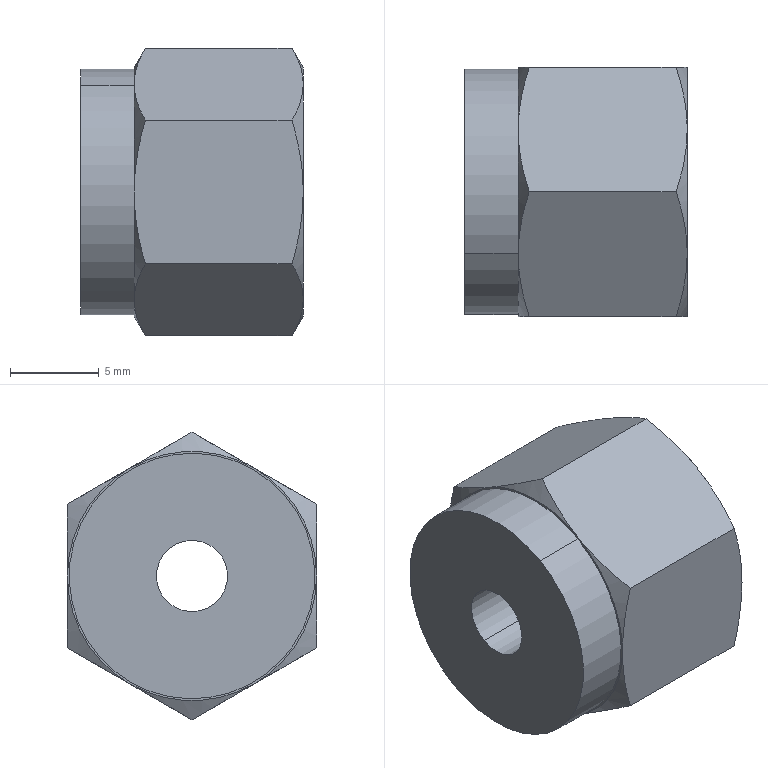Part | STEP file | SKTGK4-1-Part-1-7 | 1 solid | 28 faces | box 12.5 x 14 x 16.166 mm | volume 1459 mm3 | cone 12 | plane 10 | cylinder 6 | commonest cylinder face diameters 4 x2 11.112 x2 13.8 x2
STEP:
#1=CARTESIAN_POINT('',(7.3,9.778,3.271));
#2=VERTEX_POINT('',#1);
#3=CARTESIAN_POINT('',(7.3,4.222,12.895));
#4=VERTEX_POINT('',#3);
#5=CARTESIAN_POINT('',(7.3,7.,8.083));
#6=DIRECTION('',(1.,0.,0.));
#7=DIRECTION('',(0.,-0.5,0.866));
#8=AXIS2_PLACEMENT_3D('',#5,#6,#7);
#9=CIRCLE('',#8,5.556);
#10=EDGE_CURVE('',#2,#4,#9,.T.);
#11=ORIENTED_EDGE('',*,*,#10,.F.);
#12=CARTESIAN_POINT('',(12.5,9.778,3.271));
#13=VERTEX_POINT('',#12);
#14=CARTESIAN_POINT('',(12.5,9.778,3.271));
#15=DIRECTION('',(1.,0.,0.));
#16=VECTOR('',#15,1000.);
#17=LINE('',#14,#16);
#18=EDGE_CURVE('',#2,#13,#17,.T.);
#19=ORIENTED_EDGE('',*,*,#18,.T.);
#20=CARTESIAN_POINT('',(12.5,4.222,12.895));
#21=VERTEX_POINT('',#20);
#22=CARTESIAN_POINT('',(12.5,7.,8.083));
#23=DIRECTION('',(1.,0.,0.));
#24=DIRECTION('',(0.,-0.5,0.866));
#25=AXIS2_PLACEMENT_3D('',#22,#23,#24);
#26=CIRCLE('',#25,5.556);
#27=EDGE_CURVE('',#13,#21,#26,.T.);
#28=ORIENTED_EDGE('',*,*,#27,.T.);
#29=CARTESIAN_POINT('',(12.5,4.222,12.895));
#30=DIRECTION('',(1.,0.,0.));
#31=VECTOR('',#30,1000.);
#32=LINE('',#29,#31);
#33=EDGE_CURVE('',#4,#21,#32,.T.);
#34=ORIENTED_EDGE('',*,*,#33,.F.);
#35=EDGE_LOOP('',(#11,#19,#28,#34));
#36=FACE_OUTER_BOUND('',#35,.T.);
#37=CARTESIAN_POINT('',(12.5,7.,8.083));
#38=DIRECTION('',(1.,0.,0.));
#39=DIRECTION('',(0.,-0.5,0.866));
#40=AXIS2_PLACEMENT_3D('',#37,#38,#39);
#41=CYLINDRICAL_SURFACE('',#40,5.556);
#42=ADVANCED_FACE('',(#36),#41,.F.);
#43=CARTESIAN_POINT('',(0.,8.,6.351));
#44=VERTEX_POINT('',#43);
#45=CARTESIAN_POINT('',(0.,6.,9.815));
#46=VERTEX_POINT('',#45);
#47=CARTESIAN_POINT('',(0.,7.,8.083));
#48=DIRECTION('',(1.,0.,0.));
#49=DIRECTION('',(0.,-0.5,0.866));
#50=AXIS2_PLACEMENT_3D('',#47,#48,#49);
#51=CIRCLE('',#50,2.);
#52=EDGE_CURVE('',#44,#46,#51,.T.);
#53=ORIENTED_EDGE('',*,*,#52,.F.);
#54=CARTESIAN_POINT('',(7.3,8.,6.351));
#55=VERTEX_POINT('',#54);
#56=CARTESIAN_POINT('',(12.5,8.,6.351));
#57=DIRECTION('',(1.,0.,0.));
#58=VECTOR('',#57,1000.);
#59=LINE('',#56,#58);
#60=EDGE_CURVE('',#44,#55,#59,.T.);
#61=ORIENTED_EDGE('',*,*,#60,.T.);
#62=CARTESIAN_POINT('',(7.3,6.,9.815));
#63=VERTEX_POINT('',#62);
#64=CARTESIAN_POINT('',(7.3,7.,8.083));
#65=DIRECTION('',(1.,0.,0.));
#66=DIRECTION('',(0.,-0.5,0.866));
#67=AXIS2_PLACEMENT_3D('',#64,#65,#66);
#68=CIRCLE('',#67,2.);
#69=EDGE_CURVE('',#55,#63,#68,.T.);
#70=ORIENTED_EDGE('',*,*,#69,.T.);
#71=CARTESIAN_POINT('',(12.5,6.,9.815));
#72=DIRECTION('',(1.,0.,0.));
#73=VECTOR('',#72,1000.);
#74=LINE('',#71,#73);
#75=EDGE_CURVE('',#46,#63,#74,.T.);
#76=ORIENTED_EDGE('',*,*,#75,.F.);
#77=EDGE_LOOP('',(#53,#61,#70,#76));
#78=FACE_OUTER_BOUND('',#77,.T.);
#79=CARTESIAN_POINT('',(12.5,7.,8.083));
#80=DIRECTION('',(1.,0.,0.));
#81=DIRECTION('',(0.,-0.5,0.866));
#82=AXIS2_PLACEMENT_3D('',#79,#80,#81);
#83=CYLINDRICAL_SURFACE('',#82,2.);
#84=ADVANCED_FACE('',(#78),#83,.F.);
#85=CARTESIAN_POINT('',(0.,3.55,14.058));
#86=VERTEX_POINT('',#85);
#87=CARTESIAN_POINT('',(0.,10.45,2.107));
#88=VERTEX_POINT('',#87);
#89=CARTESIAN_POINT('',(0.,7.,8.083));
#90=DIRECTION('',(1.,0.,0.));
#91=DIRECTION('',(0.,-0.5,0.866));
#92=AXIS2_PLACEMENT_3D('',#89,#90,#91);
#93=CIRCLE('',#92,6.9);
#94=EDGE_CURVE('',#86,#88,#93,.T.);
#95=ORIENTED_EDGE('',*,*,#94,.T.);
#96=CARTESIAN_POINT('',(3.,10.45,2.107));
#97=VERTEX_POINT('',#96);
#98=CARTESIAN_POINT('',(12.5,10.45,2.107));
#99=DIRECTION('',(1.,0.,0.));
#100=VECTOR('',#99,1000.);
#101=LINE('',#98,#100);
#102=EDGE_CURVE('',#88,#97,#101,.T.);
#103=ORIENTED_EDGE('',*,*,#102,.T.);
#104=CARTESIAN_POINT('',(3.,3.55,14.058));
#105=VERTEX_POINT('',#104);
#106=CARTESIAN_POINT('',(3.,7.,8.083));
#107=DIRECTION('',(1.,0.,0.));
#108=DIRECTION('',(0.,-0.5,0.866));
#109=AXIS2_PLACEMENT_3D('',#106,#107,#108);
#110=CIRCLE('',#109,6.9);
#111=EDGE_CURVE('',#105,#97,#110,.T.);
#112=ORIENTED_EDGE('',*,*,#111,.F.);
#113=CARTESIAN_POINT('',(12.5,3.55,14.058));
#114=DIRECTION('',(1.,0.,0.));
#115=VECTOR('',#114,1000.);
#116=LINE('',#113,#115);
#117=EDGE_CURVE('',#86,#105,#116,.T.);
#118=ORIENTED_EDGE('',*,*,#117,.F.);
#119=EDGE_LOOP('',(#95,#103,#112,#118));
#120=FACE_OUTER_BOUND('',#119,.T.);
#121=CARTESIAN_POINT('',(12.5,7.,8.083));
#122=DIRECTION('',(1.,0.,0.));
#123=DIRECTION('',(0.,-0.5,0.866));
#124=AXIS2_PLACEMENT_3D('',#121,#122,#123);
#125=CYLINDRICAL_SURFACE('',#124,6.9);
#126=ADVANCED_FACE('',(#120),#125,.T.);
#127=CARTESIAN_POINT('',(11.875,14.,4.041));
#128=VERTEX_POINT('',#127);
#129=CARTESIAN_POINT('',(12.5,10.5,2.021));
#130=VERTEX_POINT('',#129);
#131=CARTESIAN_POINT('',(11.875,14.,4.041));
#132=CARTESIAN_POINT('',(12.255,12.86,3.383));
#133=CARTESIAN_POINT('',(12.5,11.699,2.713));
#134=CARTESIAN_POINT('',(12.5,10.5,2.021));
#135=B_SPLINE_CURVE_WITH_KNOTS('',3,(#131,#132,#133,#134),.UNSPECIFIED.,.F.,.F.,(4,4),(0.008823,0.01293),.UNSPECIFIED.);
#136=EDGE_CURVE('',#128,#130,#135,.T.);
#137=ORIENTED_EDGE('',*,*,#136,.F.);
#138=CARTESIAN_POINT('',(12.5,14.,8.083));
#139=VERTEX_POINT('',#138);
#140=CARTESIAN_POINT('',(12.5,14.,8.083));
#141=CARTESIAN_POINT('',(12.5,14.,7.74));
#142=CARTESIAN_POINT('',(12.485,14.,7.395));
#143=CARTESIAN_POINT('',(12.428,14.,6.714));
#144=CARTESIAN_POINT('',(12.386,14.,6.375));
#145=CARTESIAN_POINT('',(12.222,14.,5.366));
#146=CARTESIAN_POINT('',(12.065,14.,4.701));
#147=CARTESIAN_POINT('',(11.875,14.,4.041));
#148=B_SPLINE_CURVE_WITH_KNOTS('',3,(#140,#141,#142,#143,#144,#145,#146,#147),.UNSPECIFIED.,.F.,.F.,(4,2,2,4),(0.00409,0.005108,0.006127,0.008164),.UNSPECIFIED.);
#149=EDGE_CURVE('',#139,#128,#148,.T.);
#150=ORIENTED_EDGE('',*,*,#149,.F.);
#151=CARTESIAN_POINT('',(12.5,7.,8.083));
#152=DIRECTION('',(1.,0.,0.));
#153=DIRECTION('',(0.,-0.5,0.866));
#154=AXIS2_PLACEMENT_3D('',#151,#152,#153);
#155=CIRCLE('',#154,7.);
#156=EDGE_CURVE('',#130,#139,#155,.T.);
#157=ORIENTED_EDGE('',*,*,#156,.F.);
#158=EDGE_LOOP('',(#137,#150,#157));
#159=FACE_OUTER_BOUND('',#158,.T.);
#160=CARTESIAN_POINT('',(12.5,7.,8.083));
#161=DIRECTION('',(-1.,0.,0.));
#162=DIRECTION('',(0.,0.5,-0.866));
#163=AXIS2_PLACEMENT_3D('',#160,#161,#162);
#164=CONICAL_SURFACE('',#163,7.,1.047);
#165=ADVANCED_FACE('',(#159),#164,.T.);
#166=CARTESIAN_POINT('',(11.875,7.,0.));
#167=VERTEX_POINT('',#166);
#168=CARTESIAN_POINT('',(12.5,10.5,2.021));
#169=CARTESIAN_POINT('',(12.5,9.901,1.675));
#170=CARTESIAN_POINT('',(12.44,9.309,1.333));
#171=CARTESIAN_POINT('',(12.222,8.144,0.6606));
#172=CARTESIAN_POINT('',(12.065,7.569,0.3288));
#173=CARTESIAN_POINT('',(11.875,7.,0.));
#174=B_SPLINE_CURVE_WITH_KNOTS('',3,(#168,#169,#170,#171,#172,#173),.UNSPECIFIED.,.F.,.F.,(4,2,4),(0.01293,0.01499,0.01704),.UNSPECIFIED.);
#175=EDGE_CURVE('',#130,#167,#174,.T.);
#176=ORIENTED_EDGE('',*,*,#175,.F.);
#177=CARTESIAN_POINT('',(12.5,3.5,2.021));
#178=VERTEX_POINT('',#177);
#179=CARTESIAN_POINT('',(12.5,7.,8.083));
#180=DIRECTION('',(1.,0.,0.));
#181=DIRECTION('',(0.,-0.5,0.866));
#182=AXIS2_PLACEMENT_3D('',#179,#180,#181);
#183=CIRCLE('',#182,7.);
#184=EDGE_CURVE('',#178,#130,#183,.T.);
#185=ORIENTED_EDGE('',*,*,#184,.F.);
#186=CARTESIAN_POINT('',(11.875,7.,0.));
#187=CARTESIAN_POINT('',(12.066,6.427,0.3306));
#188=CARTESIAN_POINT('',(12.223,5.851,0.6635));
#189=CARTESIAN_POINT('',(12.44,4.685,1.336));
#190=CARTESIAN_POINT('',(12.5,4.096,1.676));
#191=CARTESIAN_POINT('',(12.5,3.5,2.021));
#192=B_SPLINE_CURVE_WITH_KNOTS('',3,(#186,#187,#188,#189,#190,#191),.UNSPECIFIED.,.F.,.F.,(4,2,4),(0.000000238,0.002045,0.00409),.UNSPECIFIED.);
#193=EDGE_CURVE('',#167,#178,#192,.T.);
#194=ORIENTED_EDGE('',*,*,#193,.F.);
#195=EDGE_LOOP('',(#176,#185,#194));
#196=FACE_OUTER_BOUND('',#195,.T.);
#197=CARTESIAN_POINT('',(12.5,7.,8.083));
#198=DIRECTION('',(-1.,0.,0.));
#199=DIRECTION('',(0.,0.5,-0.866));
#200=AXIS2_PLACEMENT_3D('',#197,#198,#199);
#201=CONICAL_SURFACE('',#200,7.,1.047);
#202=ADVANCED_FACE('',(#196),#201,.T.);
#203=CARTESIAN_POINT('',(11.875,0.,4.041));
#204=VERTEX_POINT('',#203);
#205=CARTESIAN_POINT('',(12.5,0.,8.083));
#206=VERTEX_POINT('',#205);
#207=CARTESIAN_POINT('',(11.875,0.,4.041));
#208=CARTESIAN_POINT('',(12.066,0.,4.703));
#209=CARTESIAN_POINT('',(12.223,0.,5.369));
#210=CARTESIAN_POINT('',(12.44,0.,6.714));
#211=CARTESIAN_POINT('',(12.5,0.,7.394));
#212=CARTESIAN_POINT('',(12.5,0.,8.083));
#213=B_SPLINE_CURVE_WITH_KNOTS('',3,(#207,#208,#209,#210,#211,#212),.UNSPECIFIED.,.F.,.F.,(4,2,4),(0.000000238,0.002045,0.00409),.UNSPECIFIED.);
#214=EDGE_CURVE('',#204,#206,#213,.T.);
#215=ORIENTED_EDGE('',*,*,#214,.F.);
#216=CARTESIAN_POINT('',(12.5,3.5,2.021));
#217=CARTESIAN_POINT('',(12.5,3.203,2.192));
#218=CARTESIAN_POINT('',(12.485,2.905,2.364));
#219=CARTESIAN_POINT('',(12.428,2.314,2.705));
#220=CARTESIAN_POINT('',(12.386,2.021,2.874));
#221=CARTESIAN_POINT('',(12.222,1.147,3.379));
#222=CARTESIAN_POINT('',(12.065,0.5711,3.712));
#223=CARTESIAN_POINT('',(11.875,0.,4.041));
#224=B_SPLINE_CURVE_WITH_KNOTS('',3,(#216,#217,#218,#219,#220,#221,#222,#223),.UNSPECIFIED.,.F.,.F.,(4,2,2,4),(0.00409,0.005108,0.006127,0.008164),.UNSPECIFIED.);
#225=EDGE_CURVE('',#178,#204,#224,.T.);
#226=ORIENTED_EDGE('',*,*,#225,.F.);
#227=CARTESIAN_POINT('',(12.5,7.,8.083));
#228=DIRECTION('',(1.,0.,0.));
#229=DIRECTION('',(0.,-0.5,0.866));
#230=AXIS2_PLACEMENT_3D('',#227,#228,#229);
#231=CIRCLE('',#230,7.);
#232=EDGE_CURVE('',#206,#178,#231,.T.);
#233=ORIENTED_EDGE('',*,*,#232,.F.);
#234=EDGE_LOOP('',(#215,#226,#233));
#235=FACE_OUTER_BOUND('',#234,.T.);
#236=CARTESIAN_POINT('',(12.5,7.,8.083));
#237=DIRECTION('',(-1.,0.,0.));
#238=DIRECTION('',(0.,0.5,-0.866));
#239=AXIS2_PLACEMENT_3D('',#236,#237,#238);
#240=CONICAL_SURFACE('',#239,7.,1.047);
#241=ADVANCED_FACE('',(#235),#240,.T.);
#242=CARTESIAN_POINT('',(11.875,0.,12.124));
#243=VERTEX_POINT('',#242);
#244=CARTESIAN_POINT('',(12.5,0.,8.083));
#245=CARTESIAN_POINT('',(12.5,0.,8.426));
#246=CARTESIAN_POINT('',(12.485,0.,8.77));
#247=CARTESIAN_POINT('',(12.428,0.,9.452));
#248=CARTESIAN_POINT('',(12.386,0.,9.79));
#249=CARTESIAN_POINT('',(12.222,0.,10.8));
#250=CARTESIAN_POINT('',(12.065,0.,11.465));
#251=CARTESIAN_POINT('',(11.875,0.,12.124));
#252=B_SPLINE_CURVE_WITH_KNOTS('',3,(#244,#245,#246,#247,#248,#249,#250,#251),.UNSPECIFIED.,.F.,.F.,(4,2,2,4),(0.00409,0.005108,0.006127,0.008164),.UNSPECIFIED.);
#253=EDGE_CURVE('',#206,#243,#252,.T.);
#254=ORIENTED_EDGE('',*,*,#253,.F.);
#255=CARTESIAN_POINT('',(12.5,3.5,14.145));
#256=VERTEX_POINT('',#255);
#257=CARTESIAN_POINT('',(12.5,7.,8.083));
#258=DIRECTION('',(1.,0.,0.));
#259=DIRECTION('',(0.,-0.5,0.866));
#260=AXIS2_PLACEMENT_3D('',#257,#258,#259);
#261=CIRCLE('',#260,7.);
#262=EDGE_CURVE('',#256,#206,#261,.T.);
#263=ORIENTED_EDGE('',*,*,#262,.F.);
#264=CARTESIAN_POINT('',(11.875,0.,12.124));
#265=CARTESIAN_POINT('',(12.255,1.14,12.783));
#266=CARTESIAN_POINT('',(12.5,2.301,13.453));
#267=CARTESIAN_POINT('',(12.5,3.5,14.145));
#268=B_SPLINE_CURVE_WITH_KNOTS('',3,(#264,#265,#266,#267),.UNSPECIFIED.,.F.,.F.,(4,4),(0.008823,0.01293),.UNSPECIFIED.);
#269=EDGE_CURVE('',#243,#256,#268,.T.);
#270=ORIENTED_EDGE('',*,*,#269,.F.);
#271=EDGE_LOOP('',(#254,#263,#270));
#272=FACE_OUTER_BOUND('',#271,.T.);
#273=CARTESIAN_POINT('',(12.5,7.,8.083));
#274=DIRECTION('',(-1.,0.,0.));
#275=DIRECTION('',(0.,0.5,-0.866));
#276=AXIS2_PLACEMENT_3D('',#273,#274,#275);
#277=CONICAL_SURFACE('',#276,7.,1.047);
#278=ADVANCED_FACE('',(#272),#277,.T.);
#279=CARTESIAN_POINT('',(11.875,7.,16.166));
#280=VERTEX_POINT('',#279);
#281=CARTESIAN_POINT('',(12.5,3.5,14.145));
#282=CARTESIAN_POINT('',(12.5,4.099,14.491));
#283=CARTESIAN_POINT('',(12.44,4.691,14.832));
#284=CARTESIAN_POINT('',(12.222,5.856,15.505));
#285=CARTESIAN_POINT('',(12.065,6.431,15.837));
#286=CARTESIAN_POINT('',(11.875,7.,16.166));
#287=B_SPLINE_CURVE_WITH_KNOTS('',3,(#281,#282,#283,#284,#285,#286),.UNSPECIFIED.,.F.,.F.,(4,2,4),(0.01293,0.01499,0.01704),.UNSPECIFIED.);
#288=EDGE_CURVE('',#256,#280,#287,.T.);
#289=ORIENTED_EDGE('',*,*,#288,.F.);
#290=CARTESIAN_POINT('',(12.5,10.5,14.145));
#291=VERTEX_POINT('',#290);
#292=CARTESIAN_POINT('',(12.5,7.,8.083));
#293=DIRECTION('',(1.,0.,0.));
#294=DIRECTION('',(0.,-0.5,0.866));
#295=AXIS2_PLACEMENT_3D('',#292,#293,#294);
#296=CIRCLE('',#295,7.);
#297=EDGE_CURVE('',#291,#256,#296,.T.);
#298=ORIENTED_EDGE('',*,*,#297,.F.);
#299=CARTESIAN_POINT('',(11.875,7.,16.166));
#300=CARTESIAN_POINT('',(12.066,7.573,15.835));
#301=CARTESIAN_POINT('',(12.223,8.149,15.502));
#302=CARTESIAN_POINT('',(12.44,9.315,14.829));
#303=CARTESIAN_POINT('',(12.5,9.904,14.489));
#304=CARTESIAN_POINT('',(12.5,10.5,14.145));
#305=B_SPLINE_CURVE_WITH_KNOTS('',3,(#299,#300,#301,#302,#303,#304),.UNSPECIFIED.,.F.,.F.,(4,2,4),(0.000000238,0.002045,0.00409),.UNSPECIFIED.);
#306=EDGE_CURVE('',#280,#291,#305,.T.);
#307=ORIENTED_EDGE('',*,*,#306,.F.);
#308=EDGE_LOOP('',(#289,#298,#307));
#309=FACE_OUTER_BOUND('',#308,.T.);
#310=CARTESIAN_POINT('',(12.5,7.,8.083));
#311=DIRECTION('',(-1.,0.,0.));
#312=DIRECTION('',(0.,0.5,-0.866));
#313=AXIS2_PLACEMENT_3D('',#310,#311,#312);
#314=CONICAL_SURFACE('',#313,7.,1.047);
#315=ADVANCED_FACE('',(#309),#314,.T.);
#316=CARTESIAN_POINT('',(3.625,0.,12.124));
#317=VERTEX_POINT('',#316);
#318=CARTESIAN_POINT('',(3.,0.,8.083));
#319=VERTEX_POINT('',#318);
#320=CARTESIAN_POINT('',(3.625,0.,12.124));
#321=CARTESIAN_POINT('',(3.434,0.,11.463));
#322=CARTESIAN_POINT('',(3.277,0.,10.797));
#323=CARTESIAN_POINT('',(3.06,0.,9.451));
#324=CARTESIAN_POINT('',(3.,0.,8.771));
#325=CARTESIAN_POINT('',(3.,0.,8.083));
#326=B_SPLINE_CURVE_WITH_KNOTS('',3,(#320,#321,#322,#323,#324,#325),.UNSPECIFIED.,.F.,.F.,(4,2,4),(0.000000238,0.002045,0.00409),.UNSPECIFIED.);
#327=EDGE_CURVE('',#317,#319,#326,.T.);
#328=ORIENTED_EDGE('',*,*,#327,.F.);
#329=CARTESIAN_POINT('',(3.,3.5,14.145));
#330=VERTEX_POINT('',#329);
#331=CARTESIAN_POINT('',(3.,3.5,14.145));
#332=CARTESIAN_POINT('',(3.,2.901,13.799));
#333=CARTESIAN_POINT('',(3.06,2.309,13.458));
#334=CARTESIAN_POINT('',(3.278,1.144,12.785));
#335=CARTESIAN_POINT('',(3.435,0.5695,12.453));
#336=CARTESIAN_POINT('',(3.625,0.,12.124));
#337=B_SPLINE_CURVE_WITH_KNOTS('',3,(#331,#332,#333,#334,#335,#336),.UNSPECIFIED.,.F.,.F.,(4,2,4),(0.01293,0.01499,0.01704),.UNSPECIFIED.);
#338=EDGE_CURVE('',#330,#317,#337,.T.);
#339=ORIENTED_EDGE('',*,*,#338,.F.);
#340=CARTESIAN_POINT('',(3.,7.,8.083));
#341=DIRECTION('',(1.,0.,0.));
#342=DIRECTION('',(0.,-0.5,0.866));
#343=AXIS2_PLACEMENT_3D('',#340,#341,#342);
#344=CIRCLE('',#343,7.);
#345=EDGE_CURVE('',#330,#319,#344,.T.);
#346=ORIENTED_EDGE('',*,*,#345,.T.);
#347=EDGE_LOOP('',(#328,#339,#346));
#348=FACE_OUTER_BOUND('',#347,.T.);
#349=CARTESIAN_POINT('',(3.808,7.,8.083));
#350=DIRECTION('',(1.,0.,0.));
#351=DIRECTION('',(0.,-0.5,0.866));
#352=AXIS2_PLACEMENT_3D('',#349,#350,#351);
#353=CONICAL_SURFACE('',#352,8.4,1.047);
#354=ADVANCED_FACE('',(#348),#353,.T.);
#355=CARTESIAN_POINT('',(3.625,0.,4.041));
#356=VERTEX_POINT('',#355);
#357=CARTESIAN_POINT('',(3.,3.5,2.021));
#358=VERTEX_POINT('',#357);
#359=CARTESIAN_POINT('',(3.625,0.,4.041));
#360=CARTESIAN_POINT('',(3.434,0.5726,3.711));
#361=CARTESIAN_POINT('',(3.277,1.149,3.378));
#362=CARTESIAN_POINT('',(3.06,2.315,2.705));
#363=CARTESIAN_POINT('',(3.,2.904,2.365));
#364=CARTESIAN_POINT('',(3.,3.5,2.021));
#365=B_SPLINE_CURVE_WITH_KNOTS('',3,(#359,#360,#361,#362,#363,#364),.UNSPECIFIED.,.F.,.F.,(4,2,4),(0.000000238,0.002045,0.00409),.UNSPECIFIED.);
#366=EDGE_CURVE('',#356,#358,#365,.T.);
#367=ORIENTED_EDGE('',*,*,#366,.F.);
#368=CARTESIAN_POINT('',(3.,0.,8.083));
#369=CARTESIAN_POINT('',(3.,0.,7.74));
#370=CARTESIAN_POINT('',(3.015,0.,7.395));
#371=CARTESIAN_POINT('',(3.072,0.,6.714));
#372=CARTESIAN_POINT('',(3.114,0.,6.375));
#373=CARTESIAN_POINT('',(3.278,0.,5.366));
#374=CARTESIAN_POINT('',(3.435,0.,4.701));
#375=CARTESIAN_POINT('',(3.625,0.,4.041));
#376=B_SPLINE_CURVE_WITH_KNOTS('',3,(#368,#369,#370,#371,#372,#373,#374,#375),.UNSPECIFIED.,.F.,.F.,(4,2,2,4),(0.00409,0.005108,0.006127,0.008164),.UNSPECIFIED.);
#377=EDGE_CURVE('',#319,#356,#376,.T.);
#378=ORIENTED_EDGE('',*,*,#377,.F.);
#379=CARTESIAN_POINT('',(3.,7.,8.083));
#380=DIRECTION('',(1.,0.,0.));
#381=DIRECTION('',(0.,-0.5,0.866));
#382=AXIS2_PLACEMENT_3D('',#379,#380,#381);
#383=CIRCLE('',#382,7.);
#384=EDGE_CURVE('',#319,#358,#383,.T.);
#385=ORIENTED_EDGE('',*,*,#384,.T.);
#386=EDGE_LOOP('',(#367,#378,#385));
#387=FACE_OUTER_BOUND('',#386,.T.);
#388=CARTESIAN_POINT('',(3.808,7.,8.083));
#389=DIRECTION('',(1.,0.,0.));
#390=DIRECTION('',(0.,-0.5,0.866));
#391=AXIS2_PLACEMENT_3D('',#388,#389,#390);
#392=CONICAL_SURFACE('',#391,8.4,1.047);
#393=ADVANCED_FACE('',(#387),#392,.T.);
#394=CARTESIAN_POINT('',(3.625,7.,0.));
#395=VERTEX_POINT('',#394);
#396=CARTESIAN_POINT('',(3.,3.5,2.021));
#397=CARTESIAN_POINT('',(3.,3.797,1.849));
#398=CARTESIAN_POINT('',(3.015,4.095,1.677));
#399=CARTESIAN_POINT('',(3.072,4.686,1.336));
#400=CARTESIAN_POINT('',(3.114,4.979,1.167));
#401=CARTESIAN_POINT('',(3.278,5.853,0.6622));
#402=CARTESIAN_POINT('',(3.435,6.429,0.3297));
#403=CARTESIAN_POINT('',(3.625,7.,0.));
#404=B_SPLINE_CURVE_WITH_KNOTS('',3,(#396,#397,#398,#399,#400,#401,#402,#403),.UNSPECIFIED.,.F.,.F.,(4,2,2,4),(0.00409,0.005108,0.006127,0.008164),.UNSPECIFIED.);
#405=EDGE_CURVE('',#358,#395,#404,.T.);
#406=ORIENTED_EDGE('',*,*,#405,.F.);
#407=CARTESIAN_POINT('',(3.,10.5,2.021));
#408=VERTEX_POINT('',#407);
#409=CARTESIAN_POINT('',(3.,7.,8.083));
#410=DIRECTION('',(1.,0.,0.));
#411=DIRECTION('',(0.,-0.5,0.866));
#412=AXIS2_PLACEMENT_3D('',#409,#410,#411);
#413=CIRCLE('',#412,7.);
#414=EDGE_CURVE('',#358,#408,#413,.T.);
#415=ORIENTED_EDGE('',*,*,#414,.T.);
#416=CARTESIAN_POINT('',(3.625,7.,0.));
#417=CARTESIAN_POINT('',(3.245,8.14,0.6583));
#418=CARTESIAN_POINT('',(3.,9.301,1.329));
#419=CARTESIAN_POINT('',(3.,10.5,2.021));
#420=B_SPLINE_CURVE_WITH_KNOTS('',3,(#416,#417,#418,#419),.UNSPECIFIED.,.F.,.F.,(4,4),(0.008823,0.01293),.UNSPECIFIED.);
#421=EDGE_CURVE('',#395,#408,#420,.T.);
#422=ORIENTED_EDGE('',*,*,#421,.F.);
#423=EDGE_LOOP('',(#406,#415,#422));
#424=FACE_OUTER_BOUND('',#423,.T.);
#425=CARTESIAN_POINT('',(3.808,7.,8.083));
#426=DIRECTION('',(1.,0.,0.));
#427=DIRECTION('',(0.,-0.5,0.866));
#428=AXIS2_PLACEMENT_3D('',#425,#426,#427);
#429=CONICAL_SURFACE('',#428,8.4,1.047);
#430=ADVANCED_FACE('',(#424),#429,.T.);
#431=CARTESIAN_POINT('',(3.625,7.,16.166));
#432=VERTEX_POINT('',#431);
#433=CARTESIAN_POINT('',(3.625,7.,16.166));
#434=CARTESIAN_POINT('',(3.245,5.86,15.507));
#435=CARTESIAN_POINT('',(3.,4.699,14.837));
#436=CARTESIAN_POINT('',(3.,3.5,14.145));
#437=B_SPLINE_CURVE_WITH_KNOTS('',3,(#433,#434,#435,#436),.UNSPECIFIED.,.F.,.F.,(4,4),(0.008823,0.01293),.UNSPECIFIED.);
#438=EDGE_CURVE('',#432,#330,#437,.T.);
#439=ORIENTED_EDGE('',*,*,#438,.F.);
#440=CARTESIAN_POINT('',(3.,10.5,14.145));
#441=VERTEX_POINT('',#440);
#442=CARTESIAN_POINT('',(3.,10.5,14.145));
#443=CARTESIAN_POINT('',(3.,10.203,14.317));
#444=CARTESIAN_POINT('',(3.015,9.905,14.489));
#445=CARTESIAN_POINT('',(3.072,9.314,14.83));
#446=CARTESIAN_POINT('',(3.114,9.021,14.999));
#447=CARTESIAN_POINT('',(3.278,8.147,15.504));
#448=CARTESIAN_POINT('',(3.435,7.571,15.836));
#449=CARTESIAN_POINT('',(3.625,7.,16.166));
#450=B_SPLINE_CURVE_WITH_KNOTS('',3,(#442,#443,#444,#445,#446,#447,#448,#449),.UNSPECIFIED.,.F.,.F.,(4,2,2,4),(0.00409,0.005108,0.006127,0.008164),.UNSPECIFIED.);
#451=EDGE_CURVE('',#441,#432,#450,.T.);
#452=ORIENTED_EDGE('',*,*,#451,.F.);
#453=CARTESIAN_POINT('',(3.,7.,8.083));
#454=DIRECTION('',(1.,0.,0.));
#455=DIRECTION('',(0.,-0.5,0.866));
#456=AXIS2_PLACEMENT_3D('',#453,#454,#455);
#457=CIRCLE('',#456,7.);
#458=EDGE_CURVE('',#441,#330,#457,.T.);
#459=ORIENTED_EDGE('',*,*,#458,.T.);
#460=EDGE_LOOP('',(#439,#452,#459));
#461=FACE_OUTER_BOUND('',#460,.T.);
#462=CARTESIAN_POINT('',(3.808,7.,8.083));
#463=DIRECTION('',(1.,0.,0.));
#464=DIRECTION('',(0.,-0.5,0.866));
#465=AXIS2_PLACEMENT_3D('',#462,#463,#464);
#466=CONICAL_SURFACE('',#465,8.4,1.047);
#467=ADVANCED_FACE('',(#461),#466,.T.);
#468=CARTESIAN_POINT('',(3.625,14.,4.041));
#469=VERTEX_POINT('',#468);
#470=CARTESIAN_POINT('',(3.,10.5,2.021));
#471=CARTESIAN_POINT('',(3.,11.099,2.367));
#472=CARTESIAN_POINT('',(3.06,11.691,2.708));
#473=CARTESIAN_POINT('',(3.278,12.856,3.381));
#474=CARTESIAN_POINT('',(3.435,13.431,3.713));
#475=CARTESIAN_POINT('',(3.625,14.,4.041));
#476=B_SPLINE_CURVE_WITH_KNOTS('',3,(#470,#471,#472,#473,#474,#475),.UNSPECIFIED.,.F.,.F.,(4,2,4),(0.01293,0.01499,0.01704),.UNSPECIFIED.);
#477=EDGE_CURVE('',#408,#469,#476,.T.);
#478=ORIENTED_EDGE('',*,*,#477,.F.);
#479=CARTESIAN_POINT('',(3.,14.,8.083));
#480=VERTEX_POINT('',#479);
#481=CARTESIAN_POINT('',(3.,7.,8.083));
#482=DIRECTION('',(1.,0.,0.));
#483=DIRECTION('',(0.,-0.5,0.866));
#484=AXIS2_PLACEMENT_3D('',#481,#482,#483);
#485=CIRCLE('',#484,7.);
#486=EDGE_CURVE('',#408,#480,#485,.T.);
#487=ORIENTED_EDGE('',*,*,#486,.T.);
#488=CARTESIAN_POINT('',(3.625,14.,4.041));
#489=CARTESIAN_POINT('',(3.434,14.,4.703));
#490=CARTESIAN_POINT('',(3.277,14.,5.369));
#491=CARTESIAN_POINT('',(3.06,14.,6.714));
#492=CARTESIAN_POINT('',(3.,14.,7.394));
#493=CARTESIAN_POINT('',(3.,14.,8.083));
#494=B_SPLINE_CURVE_WITH_KNOTS('',3,(#488,#489,#490,#491,#492,#493),.UNSPECIFIED.,.F.,.F.,(4,2,4),(0.000000238,0.002045,0.00409),.UNSPECIFIED.);
#495=EDGE_CURVE('',#469,#480,#494,.T.);
#496=ORIENTED_EDGE('',*,*,#495,.F.);
#497=EDGE_LOOP('',(#478,#487,#496));
#498=FACE_OUTER_BOUND('',#497,.T.);
#499=CARTESIAN_POINT('',(3.808,7.,8.083));
#500=DIRECTION('',(1.,0.,0.));
#501=DIRECTION('',(0.,-0.5,0.866));
#502=AXIS2_PLACEMENT_3D('',#499,#500,#501);
#503=CONICAL_SURFACE('',#502,8.4,1.047);
#504=ADVANCED_FACE('',(#498),#503,.T.);
#505=ORIENTED_EDGE('',*,*,#102,.F.);
#506=CARTESIAN_POINT('',(0.,7.,8.083));
#507=DIRECTION('',(1.,0.,0.));
#508=DIRECTION('',(0.,-0.5,0.866));
#509=AXIS2_PLACEMENT_3D('',#506,#507,#508);
#510=CIRCLE('',#509,6.9);
#511=EDGE_CURVE('',#88,#86,#510,.T.);
#512=ORIENTED_EDGE('',*,*,#511,.T.);
#513=ORIENTED_EDGE('',*,*,#117,.T.);
#514=CARTESIAN_POINT('',(3.,7.,8.083));
#515=DIRECTION('',(1.,0.,0.));
#516=DIRECTION('',(0.,-0.5,0.866));
#517=AXIS2_PLACEMENT_3D('',#514,#515,#516);
#518=CIRCLE('',#517,6.9);
#519=EDGE_CURVE('',#97,#105,#518,.T.);
#520=ORIENTED_EDGE('',*,*,#519,.F.);
#521=EDGE_LOOP('',(#505,#512,#513,#520));
#522=FACE_OUTER_BOUND('',#521,.T.);
#523=CARTESIAN_POINT('',(12.5,7.,8.083));
#524=DIRECTION('',(1.,0.,0.));
#525=DIRECTION('',(0.,-0.5,0.866));
#526=AXIS2_PLACEMENT_3D('',#523,#524,#525);
#527=CYLINDRICAL_SURFACE('',#526,6.9);
#528=ADVANCED_FACE('',(#522),#527,.T.);
#529=CARTESIAN_POINT('',(0.,7.,8.083));
#530=DIRECTION('',(1.,0.,0.));
#531=DIRECTION('',(0.,-0.5,0.866));
#532=AXIS2_PLACEMENT_3D('',#529,#530,#531);
#533=CIRCLE('',#532,2.);
#534=EDGE_CURVE('',#46,#44,#533,.T.);
#535=ORIENTED_EDGE('',*,*,#534,.T.);
#536=ORIENTED_EDGE('',*,*,#52,.T.);
#537=EDGE_LOOP('',(#535,#536));
#538=FACE_BOUND('',#537,.T.);
#539=ORIENTED_EDGE('',*,*,#94,.F.);
#540=ORIENTED_EDGE('',*,*,#511,.F.);
#541=EDGE_LOOP('',(#539,#540));
#542=FACE_OUTER_BOUND('',#541,.T.);
#543=CARTESIAN_POINT('',(0.,1.024,4.633));
#544=DIRECTION('',(-1.,0.,0.));
#545=DIRECTION('',(0.,0.5,-0.866));
#546=AXIS2_PLACEMENT_3D('',#543,#544,#545);
#547=PLANE('',#546);
#548=ADVANCED_FACE('',(#538,#542),#547,.T.);
#549=ORIENTED_EDGE('',*,*,#60,.F.);
#550=ORIENTED_EDGE('',*,*,#534,.F.);
#551=ORIENTED_EDGE('',*,*,#75,.T.);
#552=CARTESIAN_POINT('',(7.3,7.,8.083));
#553=DIRECTION('',(1.,0.,0.));
#554=DIRECTION('',(0.,-0.5,0.866));
#555=AXIS2_PLACEMENT_3D('',#552,#553,#554);
#556=CIRCLE('',#555,2.);
#557=EDGE_CURVE('',#63,#55,#556,.T.);
#558=ORIENTED_EDGE('',*,*,#557,.T.);
#559=EDGE_LOOP('',(#549,#550,#551,#558));
#560=FACE_OUTER_BOUND('',#559,.T.);
#561=CARTESIAN_POINT('',(12.5,7.,8.083));
#562=DIRECTION('',(1.,0.,0.));
#563=DIRECTION('',(0.,-0.5,0.866));
#564=AXIS2_PLACEMENT_3D('',#561,#562,#563);
#565=CYLINDRICAL_SURFACE('',#564,2.);
#566=ADVANCED_FACE('',(#560),#565,.F.);
#567=CARTESIAN_POINT('',(7.3,7.,8.083));
#568=DIRECTION('',(1.,0.,0.));
#569=DIRECTION('',(0.,-0.5,0.866));
#570=AXIS2_PLACEMENT_3D('',#567,#568,#569);
#571=CIRCLE('',#570,5.556);
#572=EDGE_CURVE('',#4,#2,#571,.T.);
#573=ORIENTED_EDGE('',*,*,#572,.T.);
#574=ORIENTED_EDGE('',*,*,#10,.T.);
#575=EDGE_LOOP('',(#573,#574));
#576=FACE_OUTER_BOUND('',#575,.T.);
#577=ORIENTED_EDGE('',*,*,#557,.F.);
#578=ORIENTED_EDGE('',*,*,#69,.F.);
#579=EDGE_LOOP('',(#577,#578));
#580=FACE_BOUND('',#579,.T.);
#581=CARTESIAN_POINT('',(7.3,5.268,7.083));
#582=DIRECTION('',(1.,0.,0.));
#583=DIRECTION('',(0.,-0.5,0.866));
#584=AXIS2_PLACEMENT_3D('',#581,#582,#583);
#585=PLANE('',#584);
#586=ADVANCED_FACE('',(#576,#580),#585,.T.);
#587=ORIENTED_EDGE('',*,*,#18,.F.);
#588=ORIENTED_EDGE('',*,*,#572,.F.);
#589=ORIENTED_EDGE('',*,*,#33,.T.);
#590=CARTESIAN_POINT('',(12.5,7.,8.083));
#591=DIRECTION('',(1.,0.,0.));
#592=DIRECTION('',(0.,-0.5,0.866));
#593=AXIS2_PLACEMENT_3D('',#590,#591,#592);
#594=CIRCLE('',#593,5.556);
#595=EDGE_CURVE('',#21,#13,#594,.T.);
#596=ORIENTED_EDGE('',*,*,#595,.T.);
#597=EDGE_LOOP('',(#587,#588,#589,#596));
#598=FACE_OUTER_BOUND('',#597,.T.);
#599=CARTESIAN_POINT('',(12.5,7.,8.083));
#600=DIRECTION('',(1.,0.,0.));
#601=DIRECTION('',(0.,-0.5,0.866));
#602=AXIS2_PLACEMENT_3D('',#599,#600,#601);
#603=CYLINDRICAL_SURFACE('',#602,5.556);
#604=ADVANCED_FACE('',(#598),#603,.F.);
#605=ORIENTED_EDGE('',*,*,#262,.T.);
#606=ORIENTED_EDGE('',*,*,#232,.T.);
#607=ORIENTED_EDGE('',*,*,#184,.T.);
#608=ORIENTED_EDGE('',*,*,#156,.T.);
#609=CARTESIAN_POINT('',(12.5,7.,8.083));
#610=DIRECTION('',(1.,0.,0.));
#611=DIRECTION('',(0.,-0.5,0.866));
#612=AXIS2_PLACEMENT_3D('',#609,#610,#611);
#613=CIRCLE('',#612,7.);
#614=EDGE_CURVE('',#139,#291,#613,.T.);
#615=ORIENTED_EDGE('',*,*,#614,.T.);
#616=ORIENTED_EDGE('',*,*,#297,.T.);
#617=EDGE_LOOP('',(#605,#606,#607,#608,#615,#616));
#618=FACE_OUTER_BOUND('',#617,.T.);
#619=ORIENTED_EDGE('',*,*,#595,.F.);
#620=ORIENTED_EDGE('',*,*,#27,.F.);
#621=EDGE_LOOP('',(#619,#620));
#622=FACE_BOUND('',#621,.T.);
#623=CARTESIAN_POINT('',(12.5,2.188,5.305));
#624=DIRECTION('',(1.,0.,0.));
#625=DIRECTION('',(0.,-0.5,0.866));
#626=AXIS2_PLACEMENT_3D('',#623,#624,#625);
#627=PLANE('',#626);
#628=ADVANCED_FACE('',(#618,#622),#627,.T.);
#629=CARTESIAN_POINT('',(11.875,14.,12.124));
#630=VERTEX_POINT('',#629);
#631=CARTESIAN_POINT('',(12.5,10.5,14.145));
#632=CARTESIAN_POINT('',(12.5,10.797,13.974));
#633=CARTESIAN_POINT('',(12.485,11.095,13.801));
#634=CARTESIAN_POINT('',(12.428,11.686,13.461));
#635=CARTESIAN_POINT('',(12.386,11.979,13.291));
#636=CARTESIAN_POINT('',(12.222,12.853,12.787));
#637=CARTESIAN_POINT('',(12.065,13.429,12.454));
#638=CARTESIAN_POINT('',(11.875,14.,12.124));
#639=B_SPLINE_CURVE_WITH_KNOTS('',3,(#631,#632,#633,#634,#635,#636,#637,#638),.UNSPECIFIED.,.F.,.F.,(4,2,2,4),(0.00409,0.005108,0.006127,0.008164),.UNSPECIFIED.);
#640=EDGE_CURVE('',#291,#630,#639,.T.);
#641=ORIENTED_EDGE('',*,*,#640,.F.);
#642=ORIENTED_EDGE('',*,*,#614,.F.);
#643=CARTESIAN_POINT('',(11.875,14.,12.124));
#644=CARTESIAN_POINT('',(12.066,14.,11.463));
#645=CARTESIAN_POINT('',(12.223,14.,10.797));
#646=CARTESIAN_POINT('',(12.44,14.,9.451));
#647=CARTESIAN_POINT('',(12.5,14.,8.771));
#648=CARTESIAN_POINT('',(12.5,14.,8.083));
#649=B_SPLINE_CURVE_WITH_KNOTS('',3,(#643,#644,#645,#646,#647,#648),.UNSPECIFIED.,.F.,.F.,(4,2,4),(0.000000238,0.002045,0.00409),.UNSPECIFIED.);
#650=EDGE_CURVE('',#630,#139,#649,.T.);
#651=ORIENTED_EDGE('',*,*,#650,.F.);
#652=EDGE_LOOP('',(#641,#642,#651));
#653=FACE_OUTER_BOUND('',#652,.T.);
#654=CARTESIAN_POINT('',(12.5,7.,8.083));
#655=DIRECTION('',(-1.,0.,0.));
#656=DIRECTION('',(0.,0.5,-0.866));
#657=AXIS2_PLACEMENT_3D('',#654,#655,#656);
#658=CONICAL_SURFACE('',#657,7.,1.047);
#659=ADVANCED_FACE('',(#653),#658,.T.);
#660=CARTESIAN_POINT('',(3.625,14.,12.124));
#661=VERTEX_POINT('',#660);
#662=CARTESIAN_POINT('',(3.625,14.,12.124));
#663=CARTESIAN_POINT('',(3.434,13.427,12.455));
#664=CARTESIAN_POINT('',(3.277,12.851,12.788));
#665=CARTESIAN_POINT('',(3.06,11.685,13.461));
#666=CARTESIAN_POINT('',(3.,11.096,13.801));
#667=CARTESIAN_POINT('',(3.,10.5,14.145));
#668=B_SPLINE_CURVE_WITH_KNOTS('',3,(#662,#663,#664,#665,#666,#667),.UNSPECIFIED.,.F.,.F.,(4,2,4),(0.000000238,0.002045,0.00409),.UNSPECIFIED.);
#669=EDGE_CURVE('',#661,#441,#668,.T.);
#670=ORIENTED_EDGE('',*,*,#669,.F.);
#671=CARTESIAN_POINT('',(3.,14.,8.083));
#672=CARTESIAN_POINT('',(3.,14.,8.426));
#673=CARTESIAN_POINT('',(3.015,14.,8.77));
#674=CARTESIAN_POINT('',(3.072,14.,9.452));
#675=CARTESIAN_POINT('',(3.114,14.,9.79));
#676=CARTESIAN_POINT('',(3.278,14.,10.8));
#677=CARTESIAN_POINT('',(3.435,14.,11.465));
#678=CARTESIAN_POINT('',(3.625,14.,12.124));
#679=B_SPLINE_CURVE_WITH_KNOTS('',3,(#671,#672,#673,#674,#675,#676,#677,#678),.UNSPECIFIED.,.F.,.F.,(4,2,2,4),(0.00409,0.005108,0.006127,0.008164),.UNSPECIFIED.);
#680=EDGE_CURVE('',#480,#661,#679,.T.);
#681=ORIENTED_EDGE('',*,*,#680,.F.);
#682=CARTESIAN_POINT('',(3.,7.,8.083));
#683=DIRECTION('',(1.,0.,0.));
#684=DIRECTION('',(0.,-0.5,0.866));
#685=AXIS2_PLACEMENT_3D('',#682,#683,#684);
#686=CIRCLE('',#685,7.);
#687=EDGE_CURVE('',#480,#441,#686,.T.);
#688=ORIENTED_EDGE('',*,*,#687,.T.);
#689=EDGE_LOOP('',(#670,#681,#688));
#690=FACE_OUTER_BOUND('',#689,.T.);
#691=CARTESIAN_POINT('',(3.808,7.,8.083));
#692=DIRECTION('',(1.,0.,0.));
#693=DIRECTION('',(0.,-0.5,0.866));
#694=AXIS2_PLACEMENT_3D('',#691,#692,#693);
#695=CONICAL_SURFACE('',#694,8.4,1.047);
#696=ADVANCED_FACE('',(#690),#695,.T.);
#697=ORIENTED_EDGE('',*,*,#111,.T.);
#698=ORIENTED_EDGE('',*,*,#519,.T.);
#699=EDGE_LOOP('',(#697,#698));
#700=FACE_BOUND('',#699,.T.);
#701=ORIENTED_EDGE('',*,*,#384,.F.);
#702=ORIENTED_EDGE('',*,*,#345,.F.);
#703=ORIENTED_EDGE('',*,*,#458,.F.);
#704=ORIENTED_EDGE('',*,*,#687,.F.);
#705=ORIENTED_EDGE('',*,*,#486,.F.);
#706=ORIENTED_EDGE('',*,*,#414,.F.);
#707=EDGE_LOOP('',(#701,#702,#703,#704,#705,#706));
#708=FACE_OUTER_BOUND('',#707,.T.);
#709=CARTESIAN_POINT('',(3.,0.9378,4.583));
#710=DIRECTION('',(-1.,0.,0.));
#711=DIRECTION('',(0.,0.5,-0.866));
#712=AXIS2_PLACEMENT_3D('',#709,#710,#711);
#713=PLANE('',#712);
#714=ADVANCED_FACE('',(#700,#708),#713,.T.);
#715=ORIENTED_EDGE('',*,*,#136,.T.);
#716=ORIENTED_EDGE('',*,*,#175,.T.);
#717=CARTESIAN_POINT('',(12.5,7.,0.));
#718=DIRECTION('',(-1.,0.,0.));
#719=VECTOR('',#718,1000.);
#720=LINE('',#717,#719);
#721=EDGE_CURVE('',#167,#395,#720,.T.);
#722=ORIENTED_EDGE('',*,*,#721,.T.);
#723=ORIENTED_EDGE('',*,*,#421,.T.);
#724=ORIENTED_EDGE('',*,*,#477,.T.);
#725=CARTESIAN_POINT('',(12.5,14.,4.041));
#726=DIRECTION('',(-1.,0.,0.));
#727=VECTOR('',#726,1000.);
#728=LINE('',#725,#727);
#729=EDGE_CURVE('',#128,#469,#728,.T.);
#730=ORIENTED_EDGE('',*,*,#729,.F.);
#731=EDGE_LOOP('',(#715,#716,#722,#723,#724,#730));
#732=FACE_OUTER_BOUND('',#731,.T.);
#733=CARTESIAN_POINT('',(12.5,7.,0.));
#734=DIRECTION('',(0.,-0.5,0.866));
#735=DIRECTION('',(-1.,0.,0.));
#736=AXIS2_PLACEMENT_3D('',#733,#734,#735);
#737=PLANE('',#736);
#738=ADVANCED_FACE('',(#732),#737,.F.);
#739=ORIENTED_EDGE('',*,*,#193,.T.);
#740=ORIENTED_EDGE('',*,*,#225,.T.);
#741=CARTESIAN_POINT('',(12.5,0.,4.041));
#742=DIRECTION('',(-1.,0.,0.));
#743=VECTOR('',#742,1000.);
#744=LINE('',#741,#743);
#745=EDGE_CURVE('',#204,#356,#744,.T.);
#746=ORIENTED_EDGE('',*,*,#745,.T.);
#747=ORIENTED_EDGE('',*,*,#366,.T.);
#748=ORIENTED_EDGE('',*,*,#405,.T.);
#749=ORIENTED_EDGE('',*,*,#721,.F.);
#750=EDGE_LOOP('',(#739,#740,#746,#747,#748,#749));
#751=FACE_OUTER_BOUND('',#750,.T.);
#752=CARTESIAN_POINT('',(12.5,0.,4.041));
#753=DIRECTION('',(0.,0.5,0.866));
#754=DIRECTION('',(0.,-0.866,0.5));
#755=AXIS2_PLACEMENT_3D('',#752,#753,#754);
#756=PLANE('',#755);
#757=ADVANCED_FACE('',(#751),#756,.F.);
#758=ORIENTED_EDGE('',*,*,#214,.T.);
#759=ORIENTED_EDGE('',*,*,#253,.T.);
#760=CARTESIAN_POINT('',(12.5,0.,12.124));
#761=DIRECTION('',(-1.,0.,0.));
#762=VECTOR('',#761,1000.);
#763=LINE('',#760,#762);
#764=EDGE_CURVE('',#243,#317,#763,.T.);
#765=ORIENTED_EDGE('',*,*,#764,.T.);
#766=ORIENTED_EDGE('',*,*,#327,.T.);
#767=ORIENTED_EDGE('',*,*,#377,.T.);
#768=ORIENTED_EDGE('',*,*,#745,.F.);
#769=EDGE_LOOP('',(#758,#759,#765,#766,#767,#768));
#770=FACE_OUTER_BOUND('',#769,.T.);
#771=CARTESIAN_POINT('',(12.5,0.,12.124));
#772=DIRECTION('',(0.,1.,0.));
#773=DIRECTION('',(0.,0.,1.));
#774=AXIS2_PLACEMENT_3D('',#771,#772,#773);
#775=PLANE('',#774);
#776=ADVANCED_FACE('',(#770),#775,.F.);
#777=ORIENTED_EDGE('',*,*,#269,.T.);
#778=ORIENTED_EDGE('',*,*,#288,.T.);
#779=CARTESIAN_POINT('',(12.5,7.,16.166));
#780=DIRECTION('',(-1.,0.,0.));
#781=VECTOR('',#780,1000.);
#782=LINE('',#779,#781);
#783=EDGE_CURVE('',#280,#432,#782,.T.);
#784=ORIENTED_EDGE('',*,*,#783,.T.);
#785=ORIENTED_EDGE('',*,*,#438,.T.);
#786=ORIENTED_EDGE('',*,*,#338,.T.);
#787=ORIENTED_EDGE('',*,*,#764,.F.);
#788=EDGE_LOOP('',(#777,#778,#784,#785,#786,#787));
#789=FACE_OUTER_BOUND('',#788,.T.);
#790=CARTESIAN_POINT('',(12.5,7.,16.166));
#791=DIRECTION('',(0.,0.5,-0.866));
#792=DIRECTION('',(1.,0.,0.));
#793=AXIS2_PLACEMENT_3D('',#790,#791,#792);
#794=PLANE('',#793);
#795=ADVANCED_FACE('',(#789),#794,.F.);
#796=ORIENTED_EDGE('',*,*,#306,.T.);
#797=ORIENTED_EDGE('',*,*,#640,.T.);
#798=CARTESIAN_POINT('',(12.5,14.,12.124));
#799=DIRECTION('',(-1.,0.,0.));
#800=VECTOR('',#799,1000.);
#801=LINE('',#798,#800);
#802=EDGE_CURVE('',#630,#661,#801,.T.);
#803=ORIENTED_EDGE('',*,*,#802,.T.);
#804=ORIENTED_EDGE('',*,*,#669,.T.);
#805=ORIENTED_EDGE('',*,*,#451,.T.);
#806=ORIENTED_EDGE('',*,*,#783,.F.);
#807=EDGE_LOOP('',(#796,#797,#803,#804,#805,#806));
#808=FACE_OUTER_BOUND('',#807,.T.);
#809=CARTESIAN_POINT('',(12.5,14.,12.124));
#810=DIRECTION('',(0.,-0.5,-0.866));
#811=DIRECTION('',(0.,0.866,-0.5));
#812=AXIS2_PLACEMENT_3D('',#809,#810,#811);
#813=PLANE('',#812);
#814=ADVANCED_FACE('',(#808),#813,.F.);
#815=ORIENTED_EDGE('',*,*,#650,.T.);
#816=ORIENTED_EDGE('',*,*,#149,.T.);
#817=ORIENTED_EDGE('',*,*,#729,.T.);
#818=ORIENTED_EDGE('',*,*,#495,.T.);
#819=ORIENTED_EDGE('',*,*,#680,.T.);
#820=ORIENTED_EDGE('',*,*,#802,.F.);
#821=EDGE_LOOP('',(#815,#816,#817,#818,#819,#820));
#822=FACE_OUTER_BOUND('',#821,.T.);
#823=CARTESIAN_POINT('',(12.5,14.,4.041));
#824=DIRECTION('',(0.,-1.,0.));
#825=DIRECTION('',(0.,0.,-1.));
#826=AXIS2_PLACEMENT_3D('',#823,#824,#825);
#827=PLANE('',#826);
#828=ADVANCED_FACE('',(#822),#827,.F.);
#829=CLOSED_SHELL('',(#42,#84,#126,#165,#202,#241,#278,#315,#354,#393,#430,#467,#504,#528,#548,#566,#586,#604,#628,#659,#696,#714,#738,#757,#776,#795,#814,#828));
#830=MANIFOLD_SOLID_BREP('',#829);
#831=CARTESIAN_POINT('',(0.,0.,0.));
#832=DIRECTION('',(0.,0.,1.));
#833=DIRECTION('',(1.,0.,0.));
#834=AXIS2_PLACEMENT_3D('',#831,#832,#833);
#835=(LENGTH_UNIT()NAMED_UNIT(*)SI_UNIT(.MILLI.,.METRE.));
#836=UNCERTAINTY_MEASURE_WITH_UNIT(LENGTH_MEASURE(0.00001),#835,'','');
#837=(NAMED_UNIT(*)PLANE_ANGLE_UNIT()SI_UNIT($,.RADIAN.));
#838=(NAMED_UNIT(*)SI_UNIT($,.STERADIAN.)SOLID_ANGLE_UNIT());
#839=(GEOMETRIC_REPRESENTATION_CONTEXT(3)GLOBAL_UNCERTAINTY_ASSIGNED_CONTEXT((#836))GLOBAL_UNIT_ASSIGNED_CONTEXT((#835,#837,#838))REPRESENTATION_CONTEXT('',''));
#840=ADVANCED_BREP_SHAPE_REPRESENTATION('',(#830,#834),#839);